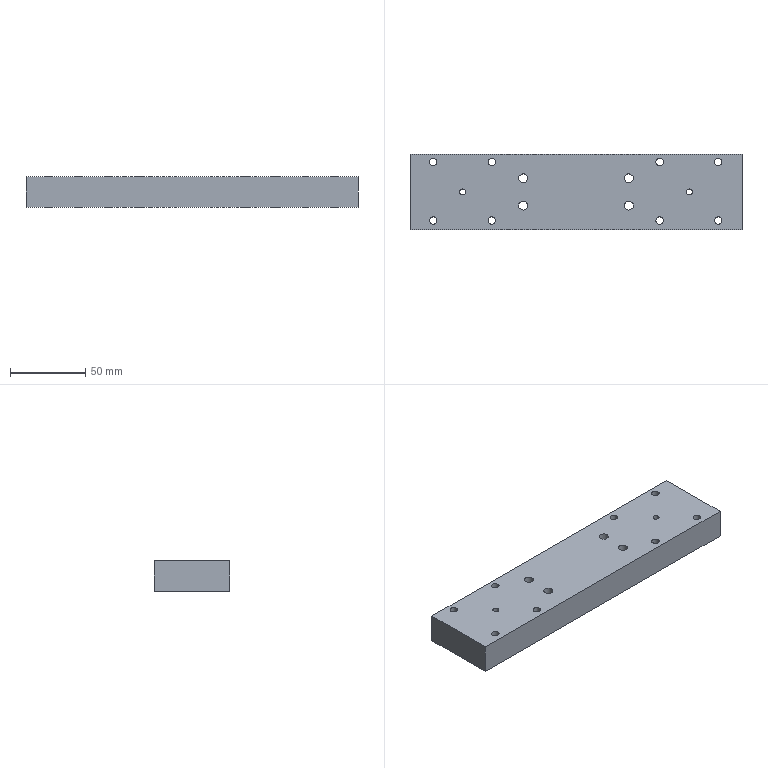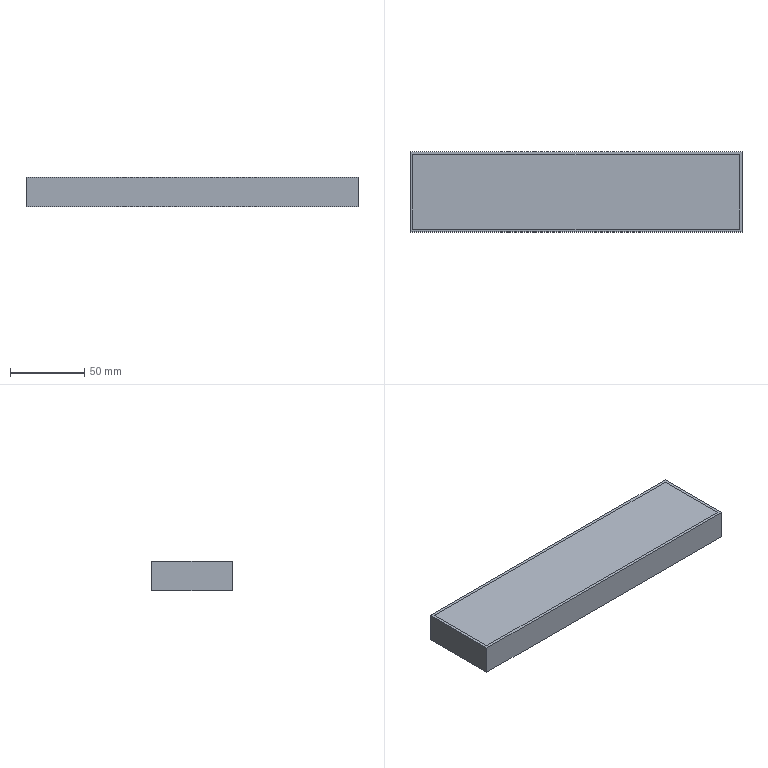CAM job | NX | 3-axis milling, drilling | part box 220 x 50 x 20 mm | stock box 224 x 54 x 20 mm
Tools:
number,name,description,diameter,corner_radius,flute_length,length,flutes
10,D10,Milling Tool-5 Parameters,10.0,0.0,50.0,75.0,2
11,D10JING,Milling Tool-5 Parameters,10.0,0.0,50.0,75.0,2
7,D6A45,Milling Tool-5 Parameters,6.0,0.0,3.0,3.0,2
16,6.0ZT,Drilling Tool,6.0,0.0,35.0,50.0,2
15,5.0ZT,Drilling Tool,5.0,0.0,35.0,50.0,2
14,3.3ZT,Drilling Tool,4.0,0.0,35.0,50.0,2
Operations:
program,operation,operation_type,tool,method,geometry_group,spindle_rpm,surface_speed,feed_per_tooth,feed_cut,feed_plunge,cut_length_mm,path_length_mm,cut_time_min,machine_time_min
1,ZLEVEL_PROFILE_1,ZLevelMilling,D10,METHOD,A,9500.0,298.0,0.1579,3000.0,100.0,15531.263,15607.963,5.177,5.185
1,ZLEVEL_PROFILE,ZLevelMilling,D10JING,METHOD,A,9500.0,298.0,0.0658,1250.0,100.0,579.754,676.354,0.4638,0.4735
1,PLANAR_MILL,PlanarMilling,D6A45,METHOD,A,9500.0,179.0,0.0658,1250.0,500.0,830.434,2105.141,0.7372,0.8647
2,DRILLING,Operation,D6A45,METHOD,B,5000.0,94.0,0.025,250.0,0.0,56.0,629.055,0.224,0.2813
2,DRILLING_COPY,Operation,6.0ZT,METHOD,B,2000.0,31.0,0.0375,150.0,0.0,105.21,385.981,0.7014,0.7295
2,DRILLING_COPY_COPY,Operation,5.0ZT,METHOD,B,2000.0,31.0,0.0375,150.0,0.0,208.017,842.222,1.387,1.45
2,DRILLING_COPY_COPY_COPY,Operation,3.3ZT,METHOD,B,2000.0,31.0,0.0375,150.0,0.0,51.403,315.837,0.3427,0.3691
2,PLANAR_MILL_COPY,PlanarMilling,D6A45,METHOD,B,9500.0,179.0,0.0658,1250.0,500.0,830.434,2107.538,0.7372,0.8649